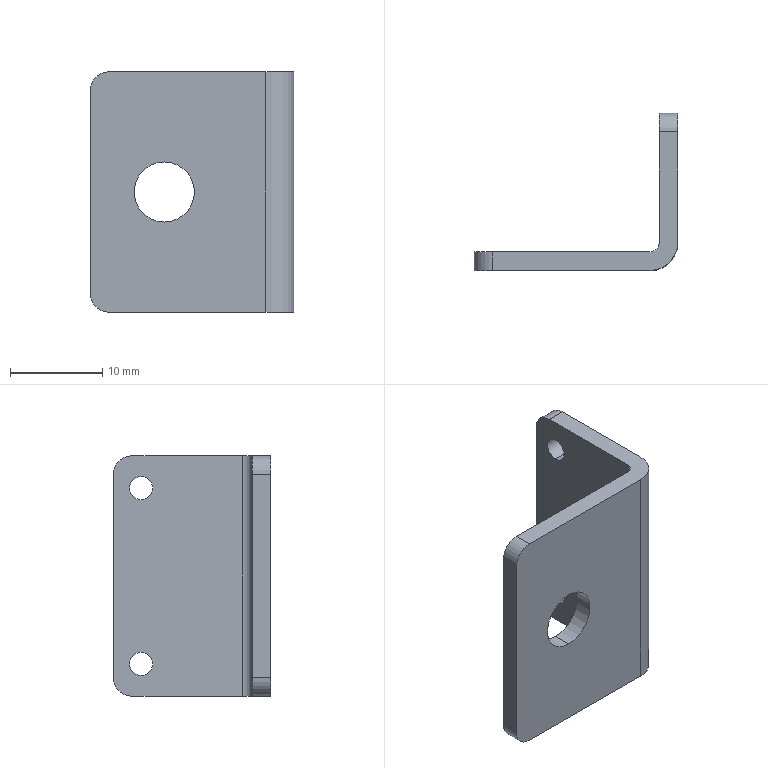Part | SolidWorks | features Fillet 3, ExtruThin 1, HoleWzd 1, ICE 1 | 1 solid | 20 faces | box 22 x 17 x 26 mm | volume 1786 mm3 | cylinder 12 | plane 8 | commonest cylinder face diameters 2.5 x4 4 x4 6.5 x2 2 x1 6 x1
STEP:
#1=CARTESIAN_POINT('',(20.,12.,21.25));
#2=VERTEX_POINT('',#1);
#3=CARTESIAN_POINT('',(20.,12.,23.75));
#4=VERTEX_POINT('',#3);
#5=CARTESIAN_POINT('',(20.,12.,22.5));
#6=DIRECTION('',(-1.,0.,0.));
#7=DIRECTION('',(0.,0.,1.));
#8=AXIS2_PLACEMENT_3D('',#5,#6,#7);
#9=CIRCLE('',#8,1.25);
#10=EDGE_CURVE('',#2,#4,#9,.T.);
#11=ORIENTED_EDGE('',*,*,#10,.T.);
#12=CARTESIAN_POINT('',(22.,12.,23.75));
#13=VERTEX_POINT('',#12);
#14=CARTESIAN_POINT('',(22.,12.,23.75));
#15=DIRECTION('',(1.,0.,0.));
#16=VECTOR('',#15,1000.);
#17=LINE('',#14,#16);
#18=EDGE_CURVE('',#4,#13,#17,.T.);
#19=ORIENTED_EDGE('',*,*,#18,.T.);
#20=CARTESIAN_POINT('',(22.,12.,21.25));
#21=VERTEX_POINT('',#20);
#22=CARTESIAN_POINT('',(22.,12.,22.5));
#23=DIRECTION('',(1.,0.,0.));
#24=DIRECTION('',(0.,0.,-1.));
#25=AXIS2_PLACEMENT_3D('',#22,#23,#24);
#26=CIRCLE('',#25,1.25);
#27=EDGE_CURVE('',#13,#21,#26,.T.);
#28=ORIENTED_EDGE('',*,*,#27,.T.);
#29=CARTESIAN_POINT('',(22.,12.,21.25));
#30=DIRECTION('',(1.,0.,0.));
#31=VECTOR('',#30,1000.);
#32=LINE('',#29,#31);
#33=EDGE_CURVE('',#2,#21,#32,.T.);
#34=ORIENTED_EDGE('',*,*,#33,.F.);
#35=EDGE_LOOP('',(#11,#19,#28,#34));
#36=FACE_OUTER_BOUND('',#35,.T.);
#37=CARTESIAN_POINT('',(22.,12.,22.5));
#38=DIRECTION('',(1.,0.,0.));
#39=DIRECTION('',(0.,0.,-1.));
#40=AXIS2_PLACEMENT_3D('',#37,#38,#39);
#41=CYLINDRICAL_SURFACE('',#40,1.25);
#42=ADVANCED_FACE('',(#36),#41,.F.);
#43=CARTESIAN_POINT('',(20.,12.,2.25));
#44=VERTEX_POINT('',#43);
#45=CARTESIAN_POINT('',(20.,12.,4.75));
#46=VERTEX_POINT('',#45);
#47=CARTESIAN_POINT('',(20.,12.,3.5));
#48=DIRECTION('',(-1.,0.,0.));
#49=DIRECTION('',(0.,0.,1.));
#50=AXIS2_PLACEMENT_3D('',#47,#48,#49);
#51=CIRCLE('',#50,1.25);
#52=EDGE_CURVE('',#44,#46,#51,.T.);
#53=ORIENTED_EDGE('',*,*,#52,.T.);
#54=CARTESIAN_POINT('',(22.,12.,4.75));
#55=VERTEX_POINT('',#54);
#56=CARTESIAN_POINT('',(22.,12.,4.75));
#57=DIRECTION('',(1.,0.,0.));
#58=VECTOR('',#57,1000.);
#59=LINE('',#56,#58);
#60=EDGE_CURVE('',#46,#55,#59,.T.);
#61=ORIENTED_EDGE('',*,*,#60,.T.);
#62=CARTESIAN_POINT('',(22.,12.,2.25));
#63=VERTEX_POINT('',#62);
#64=CARTESIAN_POINT('',(22.,12.,3.5));
#65=DIRECTION('',(1.,0.,0.));
#66=DIRECTION('',(0.,0.,-1.));
#67=AXIS2_PLACEMENT_3D('',#64,#65,#66);
#68=CIRCLE('',#67,1.25);
#69=EDGE_CURVE('',#55,#63,#68,.T.);
#70=ORIENTED_EDGE('',*,*,#69,.T.);
#71=CARTESIAN_POINT('',(22.,12.,2.25));
#72=DIRECTION('',(1.,0.,0.));
#73=VECTOR('',#72,1000.);
#74=LINE('',#71,#73);
#75=EDGE_CURVE('',#44,#63,#74,.T.);
#76=ORIENTED_EDGE('',*,*,#75,.F.);
#77=EDGE_LOOP('',(#53,#61,#70,#76));
#78=FACE_OUTER_BOUND('',#77,.T.);
#79=CARTESIAN_POINT('',(22.,12.,3.5));
#80=DIRECTION('',(1.,0.,0.));
#81=DIRECTION('',(0.,0.,-1.));
#82=AXIS2_PLACEMENT_3D('',#79,#80,#81);
#83=CYLINDRICAL_SURFACE('',#82,1.25);
#84=ADVANCED_FACE('',(#78),#83,.F.);
#85=CARTESIAN_POINT('',(8.,-2.,9.75));
#86=VERTEX_POINT('',#85);
#87=CARTESIAN_POINT('',(8.,-2.,16.25));
#88=VERTEX_POINT('',#87);
#89=CARTESIAN_POINT('',(8.,-2.,13.));
#90=DIRECTION('',(0.,1.,0.));
#91=DIRECTION('',(0.,0.,1.));
#92=AXIS2_PLACEMENT_3D('',#89,#90,#91);
#93=CIRCLE('',#92,3.25);
#94=EDGE_CURVE('',#86,#88,#93,.T.);
#95=ORIENTED_EDGE('',*,*,#94,.F.);
#96=CARTESIAN_POINT('',(8.,0.,9.75));
#97=VERTEX_POINT('',#96);
#98=CARTESIAN_POINT('',(8.,-2.,9.75));
#99=DIRECTION('',(0.,1.,0.));
#100=VECTOR('',#99,1000.);
#101=LINE('',#98,#100);
#102=EDGE_CURVE('',#86,#97,#101,.T.);
#103=ORIENTED_EDGE('',*,*,#102,.T.);
#104=CARTESIAN_POINT('',(8.,0.,16.25));
#105=VERTEX_POINT('',#104);
#106=CARTESIAN_POINT('',(8.,0.,13.));
#107=DIRECTION('',(0.,1.,0.));
#108=DIRECTION('',(0.,0.,1.));
#109=AXIS2_PLACEMENT_3D('',#106,#107,#108);
#110=CIRCLE('',#109,3.25);
#111=EDGE_CURVE('',#97,#105,#110,.T.);
#112=ORIENTED_EDGE('',*,*,#111,.T.);
#113=CARTESIAN_POINT('',(8.,-2.,16.25));
#114=DIRECTION('',(0.,1.,0.));
#115=VECTOR('',#114,1000.);
#116=LINE('',#113,#115);
#117=EDGE_CURVE('',#88,#105,#116,.T.);
#118=ORIENTED_EDGE('',*,*,#117,.F.);
#119=EDGE_LOOP('',(#95,#103,#112,#118));
#120=FACE_OUTER_BOUND('',#119,.T.);
#121=CARTESIAN_POINT('',(8.,-2.,13.));
#122=DIRECTION('',(0.,1.,0.));
#123=DIRECTION('',(0.,0.,1.));
#124=AXIS2_PLACEMENT_3D('',#121,#122,#123);
#125=CYLINDRICAL_SURFACE('',#124,3.25);
#126=ADVANCED_FACE('',(#120),#125,.F.);
#127=CARTESIAN_POINT('',(22.,12.,22.5));
#128=DIRECTION('',(1.,0.,0.));
#129=DIRECTION('',(0.,0.,-1.));
#130=AXIS2_PLACEMENT_3D('',#127,#128,#129);
#131=CIRCLE('',#130,1.25);
#132=EDGE_CURVE('',#21,#13,#131,.T.);
#133=ORIENTED_EDGE('',*,*,#132,.F.);
#134=ORIENTED_EDGE('',*,*,#27,.F.);
#135=EDGE_LOOP('',(#133,#134));
#136=FACE_BOUND('',#135,.T.);
#137=CARTESIAN_POINT('',(22.,12.,3.5));
#138=DIRECTION('',(1.,0.,0.));
#139=DIRECTION('',(0.,0.,-1.));
#140=AXIS2_PLACEMENT_3D('',#137,#138,#139);
#141=CIRCLE('',#140,1.25);
#142=EDGE_CURVE('',#63,#55,#141,.T.);
#143=ORIENTED_EDGE('',*,*,#142,.F.);
#144=ORIENTED_EDGE('',*,*,#69,.F.);
#145=EDGE_LOOP('',(#143,#144));
#146=FACE_BOUND('',#145,.T.);
#147=CARTESIAN_POINT('',(22.,1.,0.));
#148=VERTEX_POINT('',#147);
#149=CARTESIAN_POINT('',(22.,13.,0.));
#150=VERTEX_POINT('',#149);
#151=CARTESIAN_POINT('',(22.,0.,0.));
#152=DIRECTION('',(0.,1.,0.));
#153=VECTOR('',#152,1000.);
#154=LINE('',#151,#153);
#155=EDGE_CURVE('',#148,#150,#154,.T.);
#156=ORIENTED_EDGE('',*,*,#155,.T.);
#157=CARTESIAN_POINT('',(22.,15.,2.));
#158=VERTEX_POINT('',#157);
#159=CARTESIAN_POINT('',(22.,13.,2.));
#160=DIRECTION('',(1.,0.,0.));
#161=DIRECTION('',(0.,0.,1.));
#162=AXIS2_PLACEMENT_3D('',#159,#160,#161);
#163=CIRCLE('',#162,2.);
#164=EDGE_CURVE('',#150,#158,#163,.T.);
#165=ORIENTED_EDGE('',*,*,#164,.T.);
#166=CARTESIAN_POINT('',(22.,15.,24.));
#167=VERTEX_POINT('',#166);
#168=CARTESIAN_POINT('',(22.,15.,26.));
#169=DIRECTION('',(0.,0.,-1.));
#170=VECTOR('',#169,1000.);
#171=LINE('',#168,#170);
#172=EDGE_CURVE('',#167,#158,#171,.T.);
#173=ORIENTED_EDGE('',*,*,#172,.F.);
#174=CARTESIAN_POINT('',(22.,13.,26.));
#175=VERTEX_POINT('',#174);
#176=CARTESIAN_POINT('',(22.,13.,24.));
#177=DIRECTION('',(1.,0.,0.));
#178=DIRECTION('',(0.,0.,1.));
#179=AXIS2_PLACEMENT_3D('',#176,#177,#178);
#180=CIRCLE('',#179,2.);
#181=EDGE_CURVE('',#167,#175,#180,.T.);
#182=ORIENTED_EDGE('',*,*,#181,.T.);
#183=CARTESIAN_POINT('',(22.,1.,26.));
#184=VERTEX_POINT('',#183);
#185=CARTESIAN_POINT('',(22.,0.,26.));
#186=DIRECTION('',(0.,1.,0.));
#187=VECTOR('',#186,1000.);
#188=LINE('',#185,#187);
#189=EDGE_CURVE('',#184,#175,#188,.T.);
#190=ORIENTED_EDGE('',*,*,#189,.F.);
#191=CARTESIAN_POINT('',(22.,1.,26.));
#192=DIRECTION('',(0.,0.,-1.));
#193=VECTOR('',#192,1000.);
#194=LINE('',#191,#193);
#195=EDGE_CURVE('',#184,#148,#194,.T.);
#196=ORIENTED_EDGE('',*,*,#195,.T.);
#197=EDGE_LOOP('',(#156,#165,#173,#182,#190,#196));
#198=FACE_OUTER_BOUND('',#197,.T.);
#199=CARTESIAN_POINT('',(22.,0.,26.));
#200=DIRECTION('',(-1.,0.,0.));
#201=DIRECTION('',(0.,0.,1.));
#202=AXIS2_PLACEMENT_3D('',#199,#200,#201);
#203=PLANE('',#202);
#204=ADVANCED_FACE('',(#136,#146,#198),#203,.F.);
#205=ORIENTED_EDGE('',*,*,#172,.T.);
#206=CARTESIAN_POINT('',(20.,15.,2.));
#207=VERTEX_POINT('',#206);
#208=CARTESIAN_POINT('',(20.,15.,2.));
#209=DIRECTION('',(-1.,0.,0.));
#210=VECTOR('',#209,1000.);
#211=LINE('',#208,#210);
#212=EDGE_CURVE('',#158,#207,#211,.T.);
#213=ORIENTED_EDGE('',*,*,#212,.T.);
#214=CARTESIAN_POINT('',(20.,15.,24.));
#215=VERTEX_POINT('',#214);
#216=CARTESIAN_POINT('',(20.,15.,26.));
#217=DIRECTION('',(0.,0.,-1.));
#218=VECTOR('',#217,1000.);
#219=LINE('',#216,#218);
#220=EDGE_CURVE('',#215,#207,#219,.T.);
#221=ORIENTED_EDGE('',*,*,#220,.F.);
#222=CARTESIAN_POINT('',(22.,15.,24.));
#223=DIRECTION('',(1.,0.,0.));
#224=VECTOR('',#223,1000.);
#225=LINE('',#222,#224);
#226=EDGE_CURVE('',#215,#167,#225,.T.);
#227=ORIENTED_EDGE('',*,*,#226,.T.);
#228=EDGE_LOOP('',(#205,#213,#221,#227));
#229=FACE_OUTER_BOUND('',#228,.T.);
#230=CARTESIAN_POINT('',(20.,15.,26.));
#231=DIRECTION('',(0.,1.,0.));
#232=DIRECTION('',(0.,0.,1.));
#233=AXIS2_PLACEMENT_3D('',#230,#231,#232);
#234=PLANE('',#233);
#235=ADVANCED_FACE('',(#229),#234,.T.);
#236=ORIENTED_EDGE('',*,*,#10,.F.);
#237=CARTESIAN_POINT('',(20.,12.,22.5));
#238=DIRECTION('',(-1.,0.,0.));
#239=DIRECTION('',(0.,0.,1.));
#240=AXIS2_PLACEMENT_3D('',#237,#238,#239);
#241=CIRCLE('',#240,1.25);
#242=EDGE_CURVE('',#4,#2,#241,.T.);
#243=ORIENTED_EDGE('',*,*,#242,.F.);
#244=EDGE_LOOP('',(#236,#243));
#245=FACE_BOUND('',#244,.T.);
#246=ORIENTED_EDGE('',*,*,#52,.F.);
#247=CARTESIAN_POINT('',(20.,12.,3.5));
#248=DIRECTION('',(-1.,0.,0.));
#249=DIRECTION('',(0.,0.,1.));
#250=AXIS2_PLACEMENT_3D('',#247,#248,#249);
#251=CIRCLE('',#250,1.25);
#252=EDGE_CURVE('',#46,#44,#251,.T.);
#253=ORIENTED_EDGE('',*,*,#252,.F.);
#254=EDGE_LOOP('',(#246,#253));
#255=FACE_BOUND('',#254,.T.);
#256=ORIENTED_EDGE('',*,*,#220,.T.);
#257=CARTESIAN_POINT('',(20.,13.,0.));
#258=VERTEX_POINT('',#257);
#259=CARTESIAN_POINT('',(20.,13.,2.));
#260=DIRECTION('',(-1.,0.,0.));
#261=DIRECTION('',(0.,0.,1.));
#262=AXIS2_PLACEMENT_3D('',#259,#260,#261);
#263=CIRCLE('',#262,2.);
#264=EDGE_CURVE('',#207,#258,#263,.T.);
#265=ORIENTED_EDGE('',*,*,#264,.T.);
#266=CARTESIAN_POINT('',(20.,1.,0.));
#267=VERTEX_POINT('',#266);
#268=CARTESIAN_POINT('',(20.,0.,0.));
#269=DIRECTION('',(0.,1.,0.));
#270=VECTOR('',#269,1000.);
#271=LINE('',#268,#270);
#272=EDGE_CURVE('',#267,#258,#271,.T.);
#273=ORIENTED_EDGE('',*,*,#272,.F.);
#274=CARTESIAN_POINT('',(20.,1.,26.));
#275=VERTEX_POINT('',#274);
#276=CARTESIAN_POINT('',(20.,1.,26.));
#277=DIRECTION('',(0.,0.,1.));
#278=VECTOR('',#277,1000.);
#279=LINE('',#276,#278);
#280=EDGE_CURVE('',#267,#275,#279,.T.);
#281=ORIENTED_EDGE('',*,*,#280,.T.);
#282=CARTESIAN_POINT('',(20.,13.,26.));
#283=VERTEX_POINT('',#282);
#284=CARTESIAN_POINT('',(20.,0.,26.));
#285=DIRECTION('',(0.,1.,0.));
#286=VECTOR('',#285,1000.);
#287=LINE('',#284,#286);
#288=EDGE_CURVE('',#275,#283,#287,.T.);
#289=ORIENTED_EDGE('',*,*,#288,.T.);
#290=CARTESIAN_POINT('',(20.,13.,24.));
#291=DIRECTION('',(-1.,0.,0.));
#292=DIRECTION('',(0.,0.,1.));
#293=AXIS2_PLACEMENT_3D('',#290,#291,#292);
#294=CIRCLE('',#293,2.);
#295=EDGE_CURVE('',#283,#215,#294,.T.);
#296=ORIENTED_EDGE('',*,*,#295,.T.);
#297=EDGE_LOOP('',(#256,#265,#273,#281,#289,#296));
#298=FACE_OUTER_BOUND('',#297,.T.);
#299=CARTESIAN_POINT('',(20.,0.,26.));
#300=DIRECTION('',(-1.,0.,0.));
#301=DIRECTION('',(0.,0.,1.));
#302=AXIS2_PLACEMENT_3D('',#299,#300,#301);
#303=PLANE('',#302);
#304=ADVANCED_FACE('',(#245,#255,#298),#303,.T.);
#305=CARTESIAN_POINT('',(8.,0.,13.));
#306=DIRECTION('',(0.,1.,0.));
#307=DIRECTION('',(0.,0.,1.));
#308=AXIS2_PLACEMENT_3D('',#305,#306,#307);
#309=CIRCLE('',#308,3.25);
#310=EDGE_CURVE('',#105,#97,#309,.T.);
#311=ORIENTED_EDGE('',*,*,#310,.F.);
#312=ORIENTED_EDGE('',*,*,#111,.F.);
#313=EDGE_LOOP('',(#311,#312));
#314=FACE_BOUND('',#313,.T.);
#315=CARTESIAN_POINT('',(0.,0.,24.));
#316=VERTEX_POINT('',#315);
#317=CARTESIAN_POINT('',(0.,0.,2.));
#318=VERTEX_POINT('',#317);
#319=CARTESIAN_POINT('',(0.,0.,26.));
#320=DIRECTION('',(0.,0.,-1.));
#321=VECTOR('',#320,1000.);
#322=LINE('',#319,#321);
#323=EDGE_CURVE('',#316,#318,#322,.T.);
#324=ORIENTED_EDGE('',*,*,#323,.F.);
#325=CARTESIAN_POINT('',(2.,0.,26.));
#326=VERTEX_POINT('',#325);
#327=CARTESIAN_POINT('',(2.,0.,24.));
#328=DIRECTION('',(0.,1.,0.));
#329=DIRECTION('',(0.,0.,1.));
#330=AXIS2_PLACEMENT_3D('',#327,#328,#329);
#331=CIRCLE('',#330,2.);
#332=EDGE_CURVE('',#316,#326,#331,.T.);
#333=ORIENTED_EDGE('',*,*,#332,.T.);
#334=CARTESIAN_POINT('',(19.,0.,26.));
#335=VERTEX_POINT('',#334);
#336=CARTESIAN_POINT('',(0.,0.,26.));
#337=DIRECTION('',(1.,0.,0.));
#338=VECTOR('',#337,1000.);
#339=LINE('',#336,#338);
#340=EDGE_CURVE('',#326,#335,#339,.T.);
#341=ORIENTED_EDGE('',*,*,#340,.T.);
#342=CARTESIAN_POINT('',(19.,0.,0.));
#343=VERTEX_POINT('',#342);
#344=CARTESIAN_POINT('',(19.,0.,0.));
#345=DIRECTION('',(0.,0.,-1.));
#346=VECTOR('',#345,1000.);
#347=LINE('',#344,#346);
#348=EDGE_CURVE('',#335,#343,#347,.T.);
#349=ORIENTED_EDGE('',*,*,#348,.T.);
#350=CARTESIAN_POINT('',(2.,0.,0.));
#351=VERTEX_POINT('',#350);
#352=CARTESIAN_POINT('',(0.,0.,0.));
#353=DIRECTION('',(1.,0.,0.));
#354=VECTOR('',#353,1000.);
#355=LINE('',#352,#354);
#356=EDGE_CURVE('',#351,#343,#355,.T.);
#357=ORIENTED_EDGE('',*,*,#356,.F.);
#358=CARTESIAN_POINT('',(2.,0.,2.));
#359=DIRECTION('',(0.,1.,0.));
#360=DIRECTION('',(0.,0.,1.));
#361=AXIS2_PLACEMENT_3D('',#358,#359,#360);
#362=CIRCLE('',#361,2.);
#363=EDGE_CURVE('',#351,#318,#362,.T.);
#364=ORIENTED_EDGE('',*,*,#363,.T.);
#365=EDGE_LOOP('',(#324,#333,#341,#349,#357,#364));
#366=FACE_OUTER_BOUND('',#365,.T.);
#367=CARTESIAN_POINT('',(0.,0.,26.));
#368=DIRECTION('',(0.,1.,0.));
#369=DIRECTION('',(0.,0.,1.));
#370=AXIS2_PLACEMENT_3D('',#367,#368,#369);
#371=PLANE('',#370);
#372=ADVANCED_FACE('',(#314,#366),#371,.T.);
#373=CARTESIAN_POINT('',(0.,-2.,24.));
#374=VERTEX_POINT('',#373);
#375=CARTESIAN_POINT('',(0.,-2.,2.));
#376=VERTEX_POINT('',#375);
#377=CARTESIAN_POINT('',(0.,-2.,26.));
#378=DIRECTION('',(0.,0.,-1.));
#379=VECTOR('',#378,1000.);
#380=LINE('',#377,#379);
#381=EDGE_CURVE('',#374,#376,#380,.T.);
#382=ORIENTED_EDGE('',*,*,#381,.F.);
#383=CARTESIAN_POINT('',(0.,0.,24.));
#384=DIRECTION('',(0.,1.,0.));
#385=VECTOR('',#384,1000.);
#386=LINE('',#383,#385);
#387=EDGE_CURVE('',#374,#316,#386,.T.);
#388=ORIENTED_EDGE('',*,*,#387,.T.);
#389=ORIENTED_EDGE('',*,*,#323,.T.);
#390=CARTESIAN_POINT('',(0.,-2.,2.));
#391=DIRECTION('',(0.,-1.,0.));
#392=VECTOR('',#391,1000.);
#393=LINE('',#390,#392);
#394=EDGE_CURVE('',#318,#376,#393,.T.);
#395=ORIENTED_EDGE('',*,*,#394,.T.);
#396=EDGE_LOOP('',(#382,#388,#389,#395));
#397=FACE_OUTER_BOUND('',#396,.T.);
#398=CARTESIAN_POINT('',(0.,-2.,26.));
#399=DIRECTION('',(-1.,0.,0.));
#400=DIRECTION('',(0.,0.,1.));
#401=AXIS2_PLACEMENT_3D('',#398,#399,#400);
#402=PLANE('',#401);
#403=ADVANCED_FACE('',(#397),#402,.T.);
#404=CARTESIAN_POINT('',(8.,-2.,13.));
#405=DIRECTION('',(0.,1.,0.));
#406=DIRECTION('',(0.,0.,1.));
#407=AXIS2_PLACEMENT_3D('',#404,#405,#406);
#408=CIRCLE('',#407,3.25);
#409=EDGE_CURVE('',#88,#86,#408,.T.);
#410=ORIENTED_EDGE('',*,*,#409,.T.);
#411=ORIENTED_EDGE('',*,*,#94,.T.);
#412=EDGE_LOOP('',(#410,#411));
#413=FACE_BOUND('',#412,.T.);
#414=CARTESIAN_POINT('',(2.,-2.,26.));
#415=VERTEX_POINT('',#414);
#416=CARTESIAN_POINT('',(19.,-2.,26.));
#417=VERTEX_POINT('',#416);
#418=CARTESIAN_POINT('',(0.,-2.,26.));
#419=DIRECTION('',(1.,0.,0.));
#420=VECTOR('',#419,1000.);
#421=LINE('',#418,#420);
#422=EDGE_CURVE('',#415,#417,#421,.T.);
#423=ORIENTED_EDGE('',*,*,#422,.F.);
#424=CARTESIAN_POINT('',(2.,-2.,24.));
#425=DIRECTION('',(0.,-1.,0.));
#426=DIRECTION('',(0.,0.,1.));
#427=AXIS2_PLACEMENT_3D('',#424,#425,#426);
#428=CIRCLE('',#427,2.);
#429=EDGE_CURVE('',#415,#374,#428,.T.);
#430=ORIENTED_EDGE('',*,*,#429,.T.);
#431=ORIENTED_EDGE('',*,*,#381,.T.);
#432=CARTESIAN_POINT('',(2.,-2.,0.));
#433=VERTEX_POINT('',#432);
#434=CARTESIAN_POINT('',(2.,-2.,2.));
#435=DIRECTION('',(0.,-1.,0.));
#436=DIRECTION('',(0.,0.,1.));
#437=AXIS2_PLACEMENT_3D('',#434,#435,#436);
#438=CIRCLE('',#437,2.);
#439=EDGE_CURVE('',#376,#433,#438,.T.);
#440=ORIENTED_EDGE('',*,*,#439,.T.);
#441=CARTESIAN_POINT('',(19.,-2.,0.));
#442=VERTEX_POINT('',#441);
#443=CARTESIAN_POINT('',(0.,-2.,0.));
#444=DIRECTION('',(1.,0.,0.));
#445=VECTOR('',#444,1000.);
#446=LINE('',#443,#445);
#447=EDGE_CURVE('',#433,#442,#446,.T.);
#448=ORIENTED_EDGE('',*,*,#447,.T.);
#449=CARTESIAN_POINT('',(19.,-2.,26.));
#450=DIRECTION('',(0.,0.,1.));
#451=VECTOR('',#450,1000.);
#452=LINE('',#449,#451);
#453=EDGE_CURVE('',#442,#417,#452,.T.);
#454=ORIENTED_EDGE('',*,*,#453,.T.);
#455=EDGE_LOOP('',(#423,#430,#431,#440,#448,#454));
#456=FACE_OUTER_BOUND('',#455,.T.);
#457=CARTESIAN_POINT('',(0.,-2.,26.));
#458=DIRECTION('',(0.,1.,0.));
#459=DIRECTION('',(0.,0.,1.));
#460=AXIS2_PLACEMENT_3D('',#457,#458,#459);
#461=PLANE('',#460);
#462=ADVANCED_FACE('',(#413,#456),#461,.F.);
#463=ORIENTED_EDGE('',*,*,#340,.F.);
#464=CARTESIAN_POINT('',(2.,-2.,26.));
#465=DIRECTION('',(0.,-1.,0.));
#466=VECTOR('',#465,1000.);
#467=LINE('',#464,#466);
#468=EDGE_CURVE('',#326,#415,#467,.T.);
#469=ORIENTED_EDGE('',*,*,#468,.T.);
#470=ORIENTED_EDGE('',*,*,#422,.T.);
#471=CARTESIAN_POINT('',(19.,1.,26.));
#472=DIRECTION('',(0.,0.,1.));
#473=DIRECTION('',(-1.,0.,0.));
#474=AXIS2_PLACEMENT_3D('',#471,#472,#473);
#475=CIRCLE('',#474,3.);
#476=EDGE_CURVE('',#417,#184,#475,.T.);
#477=ORIENTED_EDGE('',*,*,#476,.T.);
#478=ORIENTED_EDGE('',*,*,#189,.T.);
#479=CARTESIAN_POINT('',(20.,13.,26.));
#480=DIRECTION('',(-1.,0.,0.));
#481=VECTOR('',#480,1000.);
#482=LINE('',#479,#481);
#483=EDGE_CURVE('',#175,#283,#482,.T.);
#484=ORIENTED_EDGE('',*,*,#483,.T.);
#485=ORIENTED_EDGE('',*,*,#288,.F.);
#486=CARTESIAN_POINT('',(19.,1.,26.));
#487=DIRECTION('',(0.,0.,-1.));
#488=DIRECTION('',(-1.,0.,0.));
#489=AXIS2_PLACEMENT_3D('',#486,#487,#488);
#490=CIRCLE('',#489,1.);
#491=EDGE_CURVE('',#275,#335,#490,.T.);
#492=ORIENTED_EDGE('',*,*,#491,.T.);
#493=EDGE_LOOP('',(#463,#469,#470,#477,#478,#484,#485,#492));
#494=FACE_OUTER_BOUND('',#493,.T.);
#495=CARTESIAN_POINT('',(0.,0.,26.));
#496=DIRECTION('',(0.,0.,-1.));
#497=DIRECTION('',(-1.,0.,0.));
#498=AXIS2_PLACEMENT_3D('',#495,#496,#497);
#499=PLANE('',#498);
#500=ADVANCED_FACE('',(#494),#499,.F.);
#501=ORIENTED_EDGE('',*,*,#447,.F.);
#502=CARTESIAN_POINT('',(2.,0.,0.));
#503=DIRECTION('',(0.,1.,0.));
#504=VECTOR('',#503,1000.);
#505=LINE('',#502,#504);
#506=EDGE_CURVE('',#433,#351,#505,.T.);
#507=ORIENTED_EDGE('',*,*,#506,.T.);
#508=ORIENTED_EDGE('',*,*,#356,.T.);
#509=CARTESIAN_POINT('',(19.,1.,0.));
#510=DIRECTION('',(0.,0.,1.));
#511=DIRECTION('',(-1.,0.,0.));
#512=AXIS2_PLACEMENT_3D('',#509,#510,#511);
#513=CIRCLE('',#512,1.);
#514=EDGE_CURVE('',#343,#267,#513,.T.);
#515=ORIENTED_EDGE('',*,*,#514,.T.);
#516=ORIENTED_EDGE('',*,*,#272,.T.);
#517=CARTESIAN_POINT('',(0.,13.,0.));
#518=DIRECTION('',(1.,0.,0.));
#519=VECTOR('',#518,1000.);
#520=LINE('',#517,#519);
#521=EDGE_CURVE('',#258,#150,#520,.T.);
#522=ORIENTED_EDGE('',*,*,#521,.T.);
#523=ORIENTED_EDGE('',*,*,#155,.F.);
#524=CARTESIAN_POINT('',(19.,1.,0.));
#525=DIRECTION('',(0.,0.,-1.));
#526=DIRECTION('',(-1.,0.,0.));
#527=AXIS2_PLACEMENT_3D('',#524,#525,#526);
#528=CIRCLE('',#527,3.);
#529=EDGE_CURVE('',#148,#442,#528,.T.);
#530=ORIENTED_EDGE('',*,*,#529,.T.);
#531=EDGE_LOOP('',(#501,#507,#508,#515,#516,#522,#523,#530));
#532=FACE_OUTER_BOUND('',#531,.T.);
#533=CARTESIAN_POINT('',(0.,0.,0.));
#534=DIRECTION('',(0.,0.,-1.));
#535=DIRECTION('',(-1.,0.,0.));
#536=AXIS2_PLACEMENT_3D('',#533,#534,#535);
#537=PLANE('',#536);
#538=ADVANCED_FACE('',(#532),#537,.T.);
#539=ORIENTED_EDGE('',*,*,#491,.F.);
#540=ORIENTED_EDGE('',*,*,#280,.F.);
#541=ORIENTED_EDGE('',*,*,#514,.F.);
#542=ORIENTED_EDGE('',*,*,#348,.F.);
#543=EDGE_LOOP('',(#539,#540,#541,#542));
#544=FACE_OUTER_BOUND('',#543,.T.);
#545=CARTESIAN_POINT('',(19.,1.,26.));
#546=DIRECTION('',(0.,0.,1.));
#547=DIRECTION('',(1.,0.,0.));
#548=AXIS2_PLACEMENT_3D('',#545,#546,#547);
#549=CYLINDRICAL_SURFACE('',#548,1.);
#550=ADVANCED_FACE('',(#544),#549,.F.);
#551=ORIENTED_EDGE('',*,*,#476,.F.);
#552=ORIENTED_EDGE('',*,*,#453,.F.);
#553=ORIENTED_EDGE('',*,*,#529,.F.);
#554=ORIENTED_EDGE('',*,*,#195,.F.);
#555=EDGE_LOOP('',(#551,#552,#553,#554));
#556=FACE_OUTER_BOUND('',#555,.T.);
#557=CARTESIAN_POINT('',(19.,1.,26.));
#558=DIRECTION('',(0.,0.,-1.));
#559=DIRECTION('',(-1.,0.,0.));
#560=AXIS2_PLACEMENT_3D('',#557,#558,#559);
#561=CYLINDRICAL_SURFACE('',#560,3.);
#562=ADVANCED_FACE('',(#556),#561,.T.);
#563=ORIENTED_EDGE('',*,*,#429,.F.);
#564=ORIENTED_EDGE('',*,*,#468,.F.);
#565=ORIENTED_EDGE('',*,*,#332,.F.);
#566=ORIENTED_EDGE('',*,*,#387,.F.);
#567=EDGE_LOOP('',(#563,#564,#565,#566));
#568=FACE_OUTER_BOUND('',#567,.T.);
#569=CARTESIAN_POINT('',(2.,-2.,24.));
#570=DIRECTION('',(0.,-1.,0.));
#571=DIRECTION('',(0.,0.,-1.));
#572=AXIS2_PLACEMENT_3D('',#569,#570,#571);
#573=CYLINDRICAL_SURFACE('',#572,2.);
#574=ADVANCED_FACE('',(#568),#573,.T.);
#575=ORIENTED_EDGE('',*,*,#439,.F.);
#576=ORIENTED_EDGE('',*,*,#394,.F.);
#577=ORIENTED_EDGE('',*,*,#363,.F.);
#578=ORIENTED_EDGE('',*,*,#506,.F.);
#579=EDGE_LOOP('',(#575,#576,#577,#578));
#580=FACE_OUTER_BOUND('',#579,.T.);
#581=CARTESIAN_POINT('',(2.,0.,2.));
#582=DIRECTION('',(0.,1.,0.));
#583=DIRECTION('',(0.,0.,1.));
#584=AXIS2_PLACEMENT_3D('',#581,#582,#583);
#585=CYLINDRICAL_SURFACE('',#584,2.);
#586=ADVANCED_FACE('',(#580),#585,.T.);
#587=ORIENTED_EDGE('',*,*,#264,.F.);
#588=ORIENTED_EDGE('',*,*,#212,.F.);
#589=ORIENTED_EDGE('',*,*,#164,.F.);
#590=ORIENTED_EDGE('',*,*,#521,.F.);
#591=EDGE_LOOP('',(#587,#588,#589,#590));
#592=FACE_OUTER_BOUND('',#591,.T.);
#593=CARTESIAN_POINT('',(0.,13.,2.));
#594=DIRECTION('',(1.,0.,0.));
#595=DIRECTION('',(0.,0.,-1.));
#596=AXIS2_PLACEMENT_3D('',#593,#594,#595);
#597=CYLINDRICAL_SURFACE('',#596,2.);
#598=ADVANCED_FACE('',(#592),#597,.T.);
#599=ORIENTED_EDGE('',*,*,#295,.F.);
#600=ORIENTED_EDGE('',*,*,#483,.F.);
#601=ORIENTED_EDGE('',*,*,#181,.F.);
#602=ORIENTED_EDGE('',*,*,#226,.F.);
#603=EDGE_LOOP('',(#599,#600,#601,#602));
#604=FACE_OUTER_BOUND('',#603,.T.);
#605=CARTESIAN_POINT('',(20.,13.,24.));
#606=DIRECTION('',(-1.,0.,0.));
#607=DIRECTION('',(0.,0.,1.));
#608=AXIS2_PLACEMENT_3D('',#605,#606,#607);
#609=CYLINDRICAL_SURFACE('',#608,2.);
#610=ADVANCED_FACE('',(#604),#609,.T.);
#611=ORIENTED_EDGE('',*,*,#102,.F.);
#612=ORIENTED_EDGE('',*,*,#409,.F.);
#613=ORIENTED_EDGE('',*,*,#117,.T.);
#614=ORIENTED_EDGE('',*,*,#310,.T.);
#615=EDGE_LOOP('',(#611,#612,#613,#614));
#616=FACE_OUTER_BOUND('',#615,.T.);
#617=CARTESIAN_POINT('',(8.,-2.,13.));
#618=DIRECTION('',(0.,1.,0.));
#619=DIRECTION('',(0.,0.,1.));
#620=AXIS2_PLACEMENT_3D('',#617,#618,#619);
#621=CYLINDRICAL_SURFACE('',#620,3.25);
#622=ADVANCED_FACE('',(#616),#621,.F.);
#623=ORIENTED_EDGE('',*,*,#60,.F.);
#624=ORIENTED_EDGE('',*,*,#252,.T.);
#625=ORIENTED_EDGE('',*,*,#75,.T.);
#626=ORIENTED_EDGE('',*,*,#142,.T.);
#627=EDGE_LOOP('',(#623,#624,#625,#626));
#628=FACE_OUTER_BOUND('',#627,.T.);
#629=CARTESIAN_POINT('',(22.,12.,3.5));
#630=DIRECTION('',(1.,0.,0.));
#631=DIRECTION('',(0.,0.,-1.));
#632=AXIS2_PLACEMENT_3D('',#629,#630,#631);
#633=CYLINDRICAL_SURFACE('',#632,1.25);
#634=ADVANCED_FACE('',(#628),#633,.F.);
#635=ORIENTED_EDGE('',*,*,#18,.F.);
#636=ORIENTED_EDGE('',*,*,#242,.T.);
#637=ORIENTED_EDGE('',*,*,#33,.T.);
#638=ORIENTED_EDGE('',*,*,#132,.T.);
#639=EDGE_LOOP('',(#635,#636,#637,#638));
#640=FACE_OUTER_BOUND('',#639,.T.);
#641=CARTESIAN_POINT('',(22.,12.,22.5));
#642=DIRECTION('',(1.,0.,0.));
#643=DIRECTION('',(0.,0.,-1.));
#644=AXIS2_PLACEMENT_3D('',#641,#642,#643);
#645=CYLINDRICAL_SURFACE('',#644,1.25);
#646=ADVANCED_FACE('',(#640),#645,.F.);
#647=CLOSED_SHELL('',(#42,#84,#126,#204,#235,#304,#372,#403,#462,#500,#538,#550,#562,#574,#586,#598,#610,#622,#634,#646));
#648=MANIFOLD_SOLID_BREP('',#647);
#649=CARTESIAN_POINT('',(0.,0.,0.));
#650=DIRECTION('',(0.,0.,1.));
#651=DIRECTION('',(1.,0.,0.));
#652=AXIS2_PLACEMENT_3D('',#649,#650,#651);
#653=(LENGTH_UNIT()NAMED_UNIT(*)SI_UNIT(.MILLI.,.METRE.));
#654=UNCERTAINTY_MEASURE_WITH_UNIT(LENGTH_MEASURE(0.00001),#653,'','');
#655=(NAMED_UNIT(*)PLANE_ANGLE_UNIT()SI_UNIT($,.RADIAN.));
#656=(NAMED_UNIT(*)SI_UNIT($,.STERADIAN.)SOLID_ANGLE_UNIT());
#657=(GEOMETRIC_REPRESENTATION_CONTEXT(3)GLOBAL_UNCERTAINTY_ASSIGNED_CONTEXT((#654))GLOBAL_UNIT_ASSIGNED_CONTEXT((#653,#655,#656))REPRESENTATION_CONTEXT('',''));
#658=ADVANCED_BREP_SHAPE_REPRESENTATION('',(#648,#652),#657);